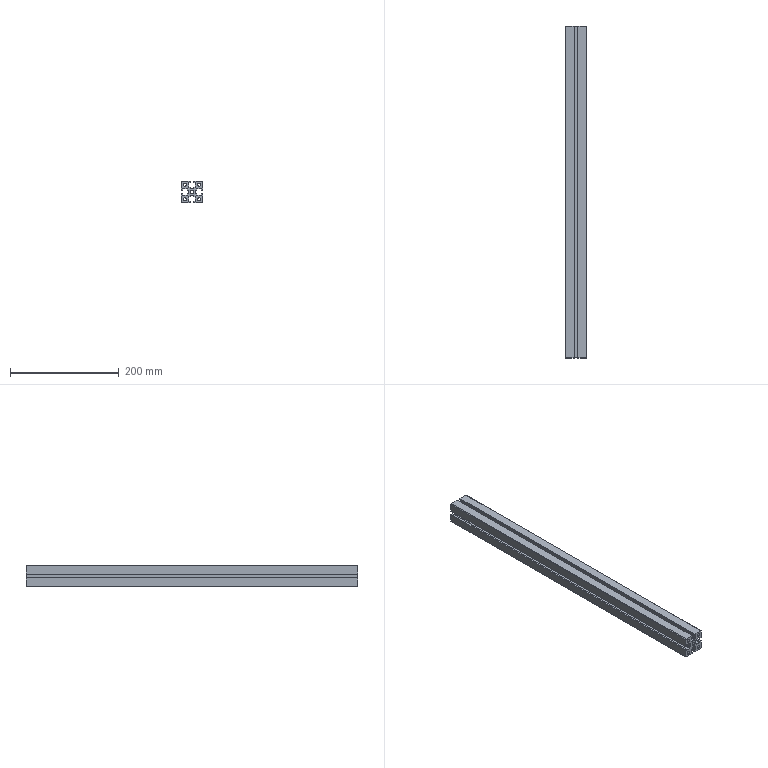Part | STEP file | 01-01 Bracket post | 1 solid | 68 faces | box 40 x 610 x 40 mm | volume 561060 mm3 | plane 54 | cylinder 14 | commonest cylinder face diameters 6 x10 2 x4